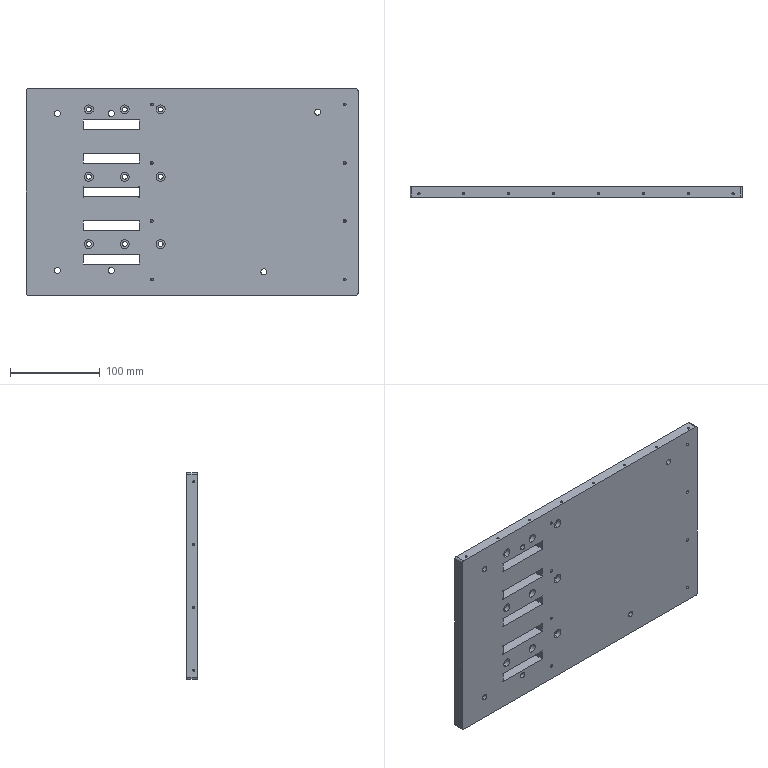Part | STEP file | GLSJ-10-27_default | 1 solid | 361 faces | box 370 x 12 x 230 mm | volume 950756 mm3 | cylinder 202 | cone 96 | plane 63 | commonest cylinder face diameters 2.5 x48 0.5 x30 5.5 x18 10 x18 3.3 x16 4.2 x16